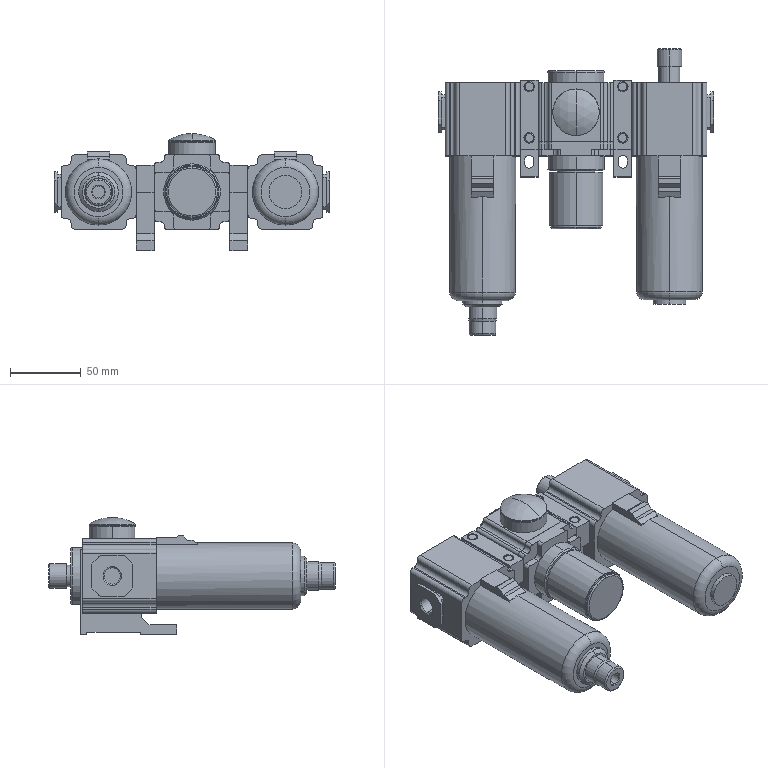Part | STEP file | GAC30008S | 5 solids | 476 faces | box 195 x 203 x 83 mm | volume 926577 mm3 | plane 281 | cylinder 141 | torus 30 | cone 22 | sphere 2 | commonest cylinder face diameters 6 x36 4 x24 11.445 x12 7 x8 7.5 x8 29.2 x8